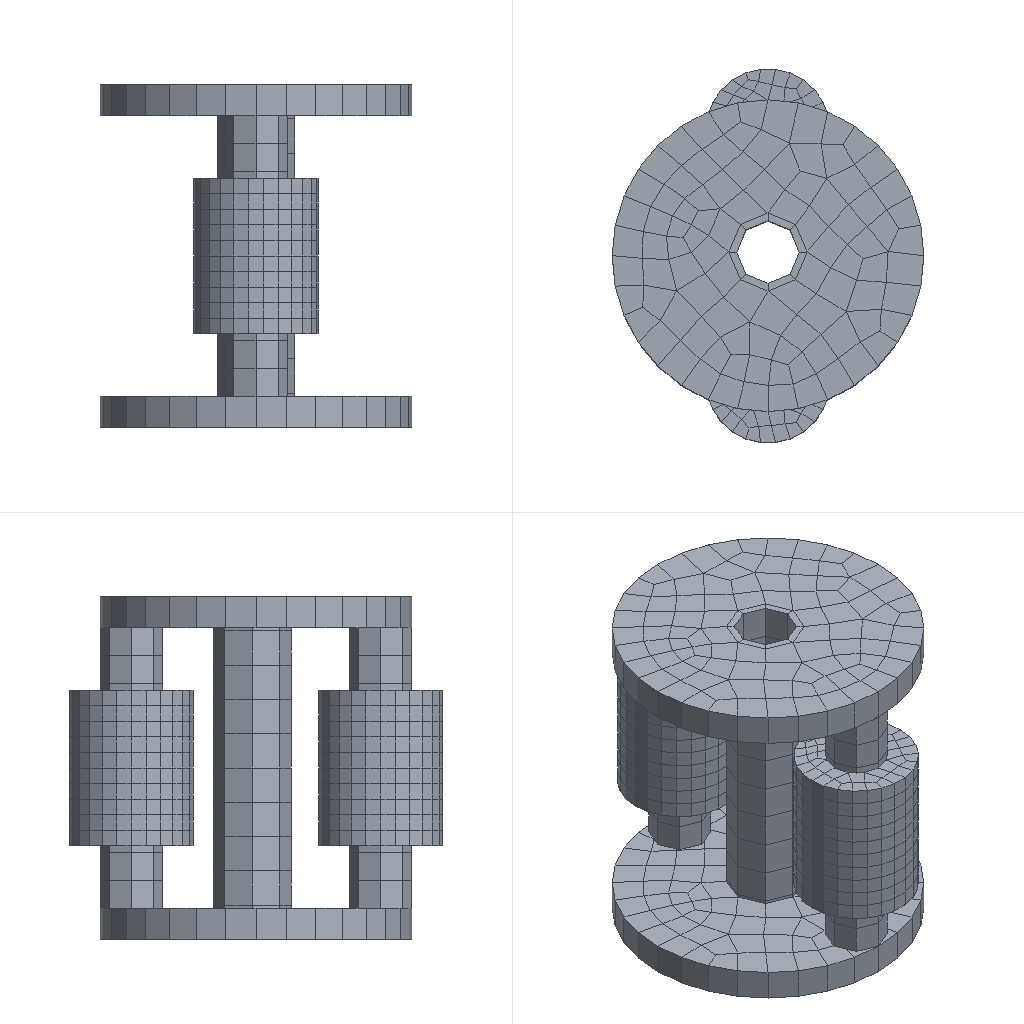Simulation study | abaqus
Set-up summary:
category,name,step,type,value,unit,region
solver,abaqus
solver,version,,,Abaqus/Explicit 2020
units,not stated in the deck,,not stated
analysis,deck,,transient,transient
load_step,Step-1,Step-1,transient
load_step,requested,,,1
mesh,nodes,,,2458
mesh,elements,,,1388
element_type,C3D8R,,solid,1388
load,load commands in deck,,count,3
bc,support commands in deck,,count,14
material,MATERIAL-1,,in results
check,setup vs results,,match,"per instance, exact: element labels, types and connectivity; labels of the nodes the elements use; coordinates not compared"
Abaqus input file, long lists of numbers shortened:
*Heading
** Job name: Job-1 Model name: Model-1
** Generated by: Abaqus/CAE 2020
*Preprint, echo=NO, model=NO, history=NO, contact=NO
**
** PARTS
**
*Part, name=duanban
*Node
      1,  -98.079,  -21.866,           0.
      2,  -92.388,   -40.626,           0.
** (226 more lines like these left out)
*Element, type=C3D8R
 1,  18, 107,  41,  17, 132, 221, 155, 131
 2,  79,  42,  94, 105, 193, 156, 208, 219
** (92 more lines like these left out)
*Nset, nset=Set-1, generate
   1,  228,    1
*Elset, elset=Set-1, generate
  1,  94,   1
** Section: Section-1
*Solid Section, elset=Set-1, material=Material-1
,
*End Part
**
*Part, name=zhuanzhou
*Node
      1,   17.678,   17.678,         120.
      2,           0.,          25.,         120.
** (174 more lines like these left out)
*Element, type=C3D8R
 1,  11,  13,   4,   8,  27,  29,  20,  24
 2,  10,  11,   8,   7,  26,  27,  24,  23
** (78 more lines like these left out)
*Nset, nset=Set-1, generate
   1,  176,    1
*Elset, elset=Set-1, generate
  1,  80,   1
** Section: Section-1
*Solid Section, elset=Set-1, material=Material-1
,
*End Part
**
*Part, name=zhuanzhou2
*Node
      1,  -14.142,  -14.142,         -90.
      2,           0.,         -20.,         -90.
** (174 more lines like these left out)
*Element, type=C3D8R
 1,   9,  12,   5,   6,  25,  28,  21,  22
 2,  10,   9,   6,   7,  26,  25,  22,  23
** (78 more lines like these left out)
*Nset, nset=Set-1, generate
   1,  176,    1
*Elset, elset=Set-1, generate
  1,  80,   1
** Section: Section-1
*Solid Section, elset=Set-1, material=Material-1
,
*End Part
**
*Part, name=zhuanzhou3
*Node
      1,  -38.838,  -9.573,         -50.
      2,  -35.418,  -18.589,         -50.
** (735 more lines like these left out)
*Element, type=C3D8R
  1,  62,  14,  15,  39, 129,  81,  82, 106
  2,  16,  40,  39,  15,  83, 107, 106,  82
** (478 more lines like these left out)
*Nset, nset=Set-1, generate
   1,  737,    1
*Elset, elset=Set-1, generate
   1,  480,    1
** Section: Section-1
*Solid Section, elset=Set-1, material=Material-1
,
*End Part
**
**
** ASSEMBLY
**
*Assembly, name=Assembly
**
*Instance, name=zhuanzhou3, part=zhuanzhou3
          0., 77.643,         110.
          0., 77.643,         110.,           0., 77.643,         111.,         180.
*End Instance
**
*Instance, name=zhuanzhou3_1, part=zhuanzhou3
          0., -82.357,         110.
          0., -82.357,         110.,           0., -82.357,         111.,         180.
*End Instance
**
*Instance, name=zhuanzhou2, part=zhuanzhou2
          0., 77.643,         110.
*End Instance
**
*Instance, name=duanban, part=duanban
          0.,           0.,         200.
*End Instance
**
*Instance, name=zhuanzhou2_2, part=zhuanzhou2
          0., -82.357,         110.
*End Instance
**
*Instance, name=zhuanzhou, part=zhuanzhou
          0.,           0.,         100.
*End Instance
**
*Instance, name=duanban_3, part=duanban
*End Instance
**
*Node
      1,           0.,           0.,         110.
*Node
      2,           0.,    77.643,         110.
*Node
      3,           0.,   -82.357,         110.
*Nset, nset=Set-5
 2, 3
*Nset, nset=Set-6
 1,
*Nset, nset=Set-7
 3,
*Nset, nset=Set-8
 2,
*Nset, nset=m_Set-1
 1,
*Nset, nset=m_Set-2
 1,
*Nset, nset=m_Set-3
 2,
*Nset, nset=m_Set-4
 3,
*Elset, elset=_m_Surf-3_S1, internal, instance=duanban, generate
  1,  94,   1
*Elset, elset=_m_Surf-3_S2, internal, instance=duanban_3, generate
  1,  94,   1
*Surface, type=ELEMENT, name=m_Surf-3
_m_Surf-3_S1, S1
_m_Surf-3_S2, S2
*Elset, elset=_s_Surf-1_S3, internal, instance=zhuanzhou
  1,  2,  3,  5,  6,  9, 10, 11, 13, 14, 17, 18, 19, 21, 22, 25
 26, 27, 29, 30, 33, 34, 35, 37, 38, 41, 42, 43, 45, 46, 49, 50
** (2 more lines like these left out)
*Elset, elset=_s_Surf-1_S5, internal, instance=zhuanzhou
  4,  7,  8, 12, 15, 16, 20, 23, 24, 28, 31, 32, 36, 39, 40, 44
 47, 48, 52, 55, 56, 60, 63, 64, 68, 71, 72, 76, 79, 80
*Surface, type=ELEMENT, name=s_Surf-1
_s_Surf-1_S3, S3
_s_Surf-1_S5, S5
*Elset, elset=_s_Surf-2_S4, internal, instance=duanban
 33, 57, 68, 71
*Elset, elset=_s_Surf-2_S4, internal, instance=duanban_3
 33, 57, 68, 71
*Elset, elset=_s_Surf-2_S3, internal, instance=duanban
 38,
*Elset, elset=_s_Surf-2_S3, internal, instance=duanban_3
 38,
*Elset, elset=_s_Surf-2_S5, internal, instance=duanban
 43, 51, 62
*Elset, elset=_s_Surf-2_S5, internal, instance=duanban_3
 43, 51, 62
*Surface, type=ELEMENT, name=s_Surf-2
_s_Surf-2_S4, S4
_s_Surf-2_S3, S3
_s_Surf-2_S5, S5
*Elset, elset=_s_Surf-3_S2, internal, instance=zhuanzhou2, generate
 73,  80,   1
*Elset, elset=_s_Surf-3_S2, internal, instance=zhuanzhou2_2, generate
 73,  80,   1
*Elset, elset=_s_Surf-3_S1, internal, instance=zhuanzhou2, generate
 1,  8,  1
*Elset, elset=_s_Surf-3_S1, internal, instance=zhuanzhou2_2, generate
 1,  8,  1
*Surface, type=ELEMENT, name=s_Surf-3
_s_Surf-3_S2, S2
_s_Surf-3_S1, S1
*Elset, elset=_s_Surf-5_S5, internal, instance=zhuanzhou3
   3,  36,  38,  41,  43,  44,  51,  84,  86,  89,  91,  92,  99, 132, 134, 137
 139, 140, 147, 180, 182, 185, 187, 188, 195, 228, 230, 233, 235, 236, 243, 276
** (2 more lines like these left out)
*Elset, elset=_s_Surf-5_S6, internal, instance=zhuanzhou3
  12,  17,  29,  39,  60,  65,  77,  87, 108, 113, 125, 135, 156, 161, 173, 183
 204, 209, 221, 231, 252, 257, 269, 279, 300, 305, 317, 327, 348, 353, 365, 375
** (1 more lines like these left out)
*Elset, elset=_s_Surf-5_S3, internal, instance=zhuanzhou3, generate
  33,  465,   48
*Elset, elset=_s_Surf-5_S4, internal, instance=zhuanzhou3, generate
  37,  469,   48
*Surface, type=ELEMENT, name=s_Surf-5
_s_Surf-5_S5, S5
_s_Surf-5_S6, S6
_s_Surf-5_S4, S4
_s_Surf-5_S3, S3
*Elset, elset=_s_Surf-6_S5, internal, instance=zhuanzhou3_1
   3,  36,  38,  41,  43,  44,  51,  84,  86,  89,  91,  92,  99, 132, 134, 137
 139, 140, 147, 180, 182, 185, 187, 188, 195, 228, 230, 233, 235, 236, 243, 276
** (2 more lines like these left out)
*Elset, elset=_s_Surf-6_S6, internal, instance=zhuanzhou3_1
  12,  17,  29,  39,  60,  65,  77,  87, 108, 113, 125, 135, 156, 161, 173, 183
 204, 209, 221, 231, 252, 257, 269, 279, 300, 305, 317, 327, 348, 353, 365, 375
** (1 more lines like these left out)
*Elset, elset=_s_Surf-6_S3, internal, instance=zhuanzhou3_1, generate
  33,  465,   48
*Elset, elset=_s_Surf-6_S4, internal, instance=zhuanzhou3_1, generate
  37,  469,   48
*Surface, type=ELEMENT, name=s_Surf-6
_s_Surf-6_S5, S5
_s_Surf-6_S6, S6
_s_Surf-6_S4, S4
_s_Surf-6_S3, S3
*Nset, nset="_T-Datum csys-2", internal
Set-7,
*Transform, nset="_T-Datum csys-2"
          1., -3.67058703432122e-09,           0., 3.67058703432122e-09,           1.,           0.
*Nset, nset="_T-Datum csys-3", internal
Set-8,
*Transform, nset="_T-Datum csys-3"
          1., -3.67058454742164e-09,           0., -3.67058454742164e-09,          -1.,           0.
** Constraint: Constraint-1
*Coupling, constraint name=Constraint-1, ref node=m_Set-1, surface=s_Surf-1
*Kinematic
** Constraint: Constraint-2
*Coupling, constraint name=Constraint-2, ref node=m_Set-2, surface=s_Surf-2
*Kinematic
** Constraint: Constraint-3
*Tie, name=Constraint-3, adjust=yes
s_Surf-3, m_Surf-3
** Constraint: Constraint-4
*Coupling, constraint name=Constraint-4, ref node=m_Set-3, surface=s_Surf-5
*Kinematic
** Constraint: Constraint-5
*Coupling, constraint name=Constraint-5, ref node=m_Set-4, surface=s_Surf-6
*Kinematic
*End Assembly
**
** MATERIALS
**
*Material, name=Material-1
*Density
 7.8e-09,
*Elastic
210000., 0.3
**
** INTERACTION PROPERTIES
**
*Surface Interaction, name=IntProp-1
*Friction
 0.2,
*Surface Behavior, pressure-overclosure=HARD
** ----------------------------------------------------------------
**
** STEP: Step-1
**
*Step, name=Step-1, nlgeom=YES
*Dynamic, Explicit
, 0.01
*Bulk Viscosity
0.06, 1.2
**
** BOUNDARY CONDITIONS
**
** Name: BC-1 Type: 速度/角速度
*Boundary, type=VELOCITY
Set-7, 3, 3
Set-7, 4, 4
Set-7, 5, 5
Set-7, 6, 6, 31.4
** Name: BC-1-Copy Type: 速度/角速度
*Boundary, type=VELOCITY
Set-8, 3, 3
Set-8, 4, 4
Set-8, 5, 5
Set-8, 6, 6, 31.4
** Name: BC-2 Type: 速度/角速度
*Boundary, type=VELOCITY
Set-6, 1, 1
Set-6, 2, 2
Set-6, 3, 3
Set-6, 4, 4
Set-6, 5, 5
Set-6, 6, 6, 15.
**
** INTERACTIONS
**
** Interaction: Int-1
*Contact, op=NEW
*Contact Inclusions, ALL EXTERIOR
*Contact Property Assignment
 ,  , IntProp-1
**
** OUTPUT REQUESTS
**
*Restart, write, number interval=1, time marks=NO
**
** FIELD OUTPUT: F-Output-1
**
*Output, field, number interval=50
*Node Output
A, AR, AT, CF, RF, U, UR, UT
V, VR, VT
*Element Output, directions=YES
E, LE, MISES, PE, PEEQ, PEMAG, S
*Contact Output
CDISP, CSTRESS
**
** HISTORY OUTPUT: H-Output-1
**
*Output, history, variable=PRESELECT, frequency=10
*End Step
Results summary:
result,step,Step-1,completed,increments=14908 time=0.01/0.01
result,analysis,,,transient
result,last_loadstep,,,1
result,primary field,,,U
result,reaction total,,FX,-9529.975,model units
result,reaction total,,FY,-2952.977,model units
result,reaction total,,FZ,389.819,model units